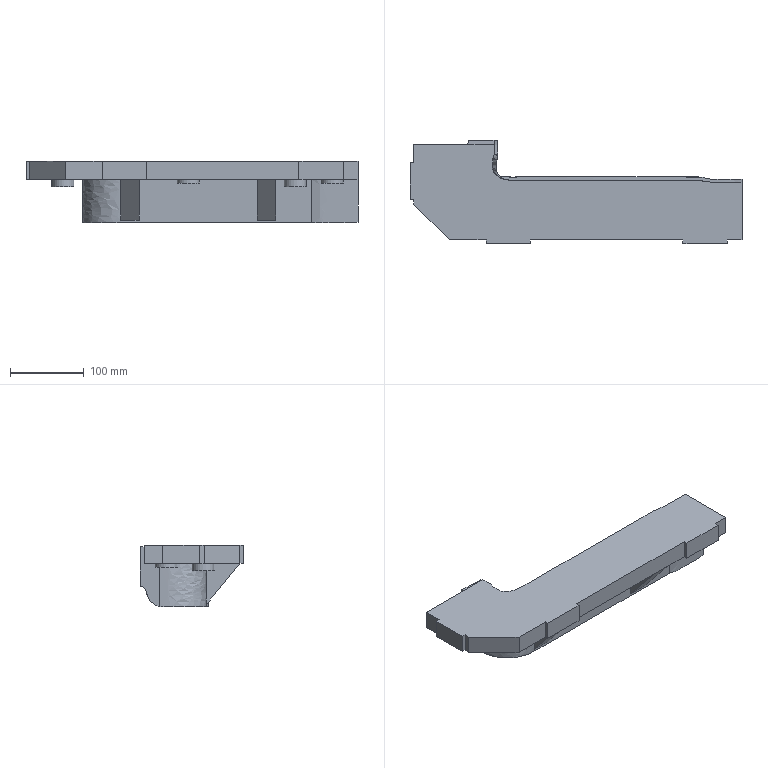Part | NX | features solid 2 | 1 solid | 87 faces | box 450 x 140 x 83.908 mm | volume 2036187 mm3 | spline 49 | plane 33 | cylinder 5 | commonest cylinder face diameters 30 x5